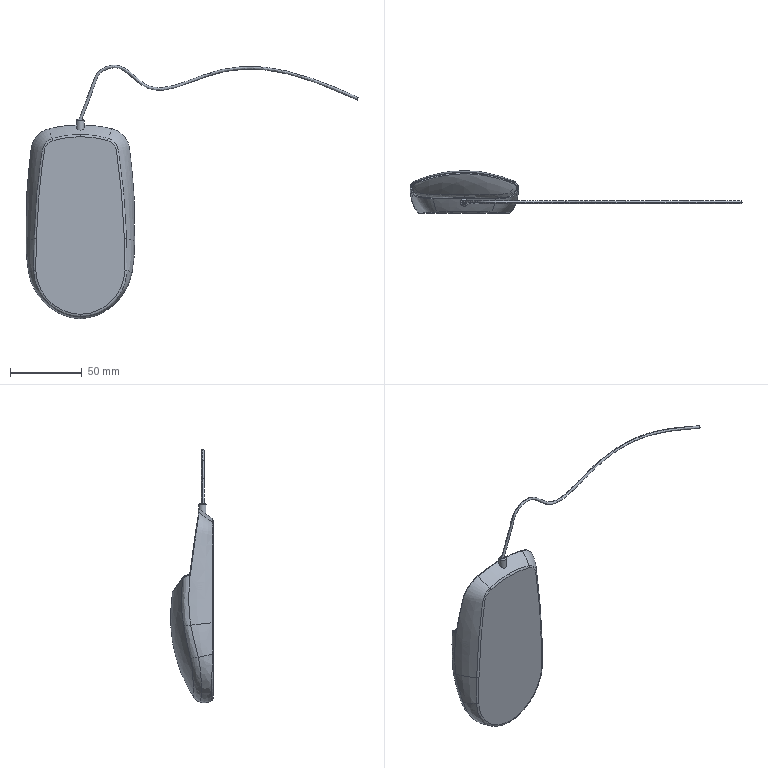Part | STEP file | Guide wheel mechanism revised.sldasm-Part-311 | 1 solid | 79 faces | box 231.61 x 29.722 x 176.987 mm | volume 19601 mm3 | spline 70 | plane 5 | cylinder 4 | commonest cylinder face diameters 5.256 x4